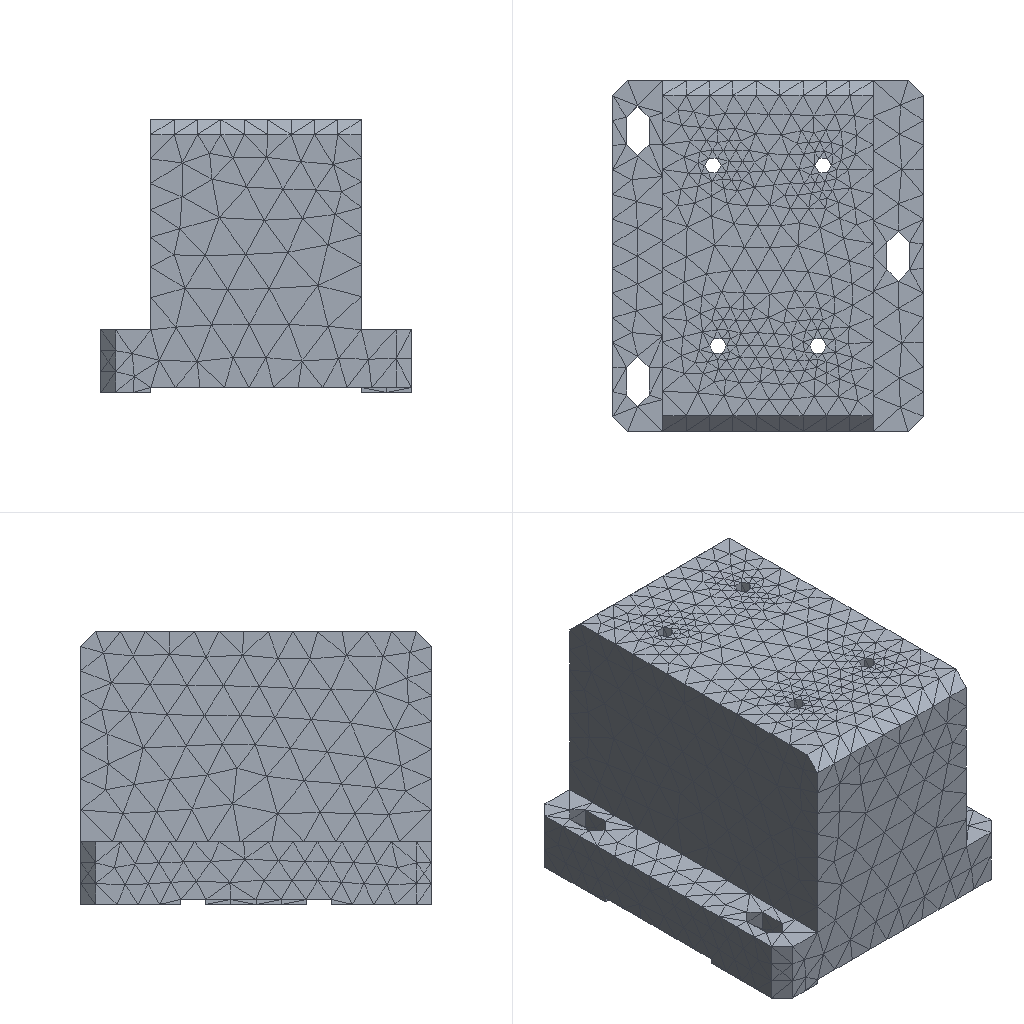Simulation study | nx simcenter
Set-up summary:
category,name,step,type,value,unit,region
solver,nx_nastran (Simcenter)
units,not stated in the deck,,not stated
analysis,deck,,static,static
analysis,solution,,SOL,101
load_step,SUBCASE 1,1,SUBCASE,SPC=1 LOAD=2
load_step,requested,,,1
mesh,nodes,,,9372
mesh,elements,,,4867
element_type,CTETRA,,solid,4867
load,nodal force total,,FX,0.0,model units
load,nodal force total,,FY,0.0,model units
load,nodal force total,,FZ,-3000000.07,model units
load,load commands in deck,,count,796
bc,support commands in deck,,count,204
analysis,NX solution 0,,Structural,Linear Statics - Single Constraint
check,setup vs results,,match,every grid point's frame and coordinates and every element id; grid points of CTETRA elements
Nastran input file, long lists of numbers shortened:
$*$$$$$$$$$$$$$$$$$$$$$$$$$$$$$$$$$$$$$$$$$$$$$$$$$$$$$$$$$$$$$$$$$
$*
$*                    NX v10.0.0.24 TRANSLATOR
$*                    FOR NX NASTRAN VERSION 10.0
$ (33 more lines like these left out)
ASSIGN OUTPUT2='131_sim1-solution_1.op2' UNIT=12
$*
$*$$$$$$$$$$$$$$$$$$$$$$$$$$$$$$$$$$$
$*
$* EXECUTIVE CONTROL
$*
$*$$$$$$$$$$$$$$$$$$$$$$$$$$$$$$$$$$$
$*
ID,NASTRAN,131_sim1-solution_1
SOL 101
CEND
$*
$*$$$$$$$$$$$$$$$$$$$$$$$$$$$$$$$$$$$
$*
$* CASE CONTROL
$*
$*$$$$$$$$$$$$$$$$$$$$$$$$$$$$$$$$$$$
$*
TITLE = Solution 1
ECHO = NONE
SPC = 1
OUTPUT
BCRESULTS(TRACTION,FORCE,PLOT) = ALL
DISPLACEMENT(PLOT) = ALL
ESE(PLOT) = ALL
FORCE(PLOT,CORNER) = ALL
OLOAD(PLOT) = ALL
SPCFORCES(PLOT) = ALL
STRAIN(PLOT,FIBER,CORNER) = ALL
STRESS(PLOT,CORNER) = ALL
$*  NX Step: Subcase - Static Loads 1
SUBCASE 1
LABEL = Subcase - Static Loads 1
LOAD = 2
$*
$*$$$$$$$$$$$$$$$$$$$$$$$$$$$$$$$$$$$
$*
$* BULK DATA
$*
$*$$$$$$$$$$$$$$$$$$$$$$$$$$$$$$$$$$$
$*
BEGIN BULK
$*
$* PARAM CARDS
$*
PARAM      K6ROT100.0000
PARAM     OIBULK     YES
PARAM    OMACHPR     YES
PARAM       POST      -2
PARAM    POSTEXT     YES
PARAM    UNITSYS   MN-MM
$*
$* GRID CARDS
$*
GRID*               9277               00.0000000000E+003.0000000000E+00+
*       0.0000000000E+00               0
GRID*               9278               0-7.234460969E-153.0000000000E+00+
*       1.2500000000E+01               0
$ (18740 more lines like these left out)
$*
$* ELEMENT CARDS
$*
$*  NX Mesh Collector: Solid(1)
$*  NX Mesh: 3d_mesh(1)
CTETRA         1       1       1       2    6003    6053     158     159+
+            160     161     162    6330
CTETRA         2       1       1       3    6003       4     163     164+
+            160     165     166     167
$ (9730 more lines like these left out)
$*
$* PROPERTY CARDS
$*
$*  NX Property: PSOLID1
PSOLID         1       1       0                           SMECH
$*
$* MATERIAL CARDS
$*
$*  NX Material: Aluminum_5086
MAT1           17.2000+7        0.3300002.6600-62.5000-5
$*
$* LOAD AND CONSTRAINT CARDS
$*
$*  NX Load and Constraint: Fixed(1)
SPC            1    4102  123456  0.0000
SPC            1    4103  123456  0.0000
SPC            1    4104  123456  0.0000
SPC            1    4105  123456  0.0000
$ (200 more lines like these left out)
$*  NX Load and Constraint: Force(1)
FORCE          2    6220       0842.4065  0.0000  0.0000-1.00000
FORCE          2    6221       0790.7649  0.0000  0.0000-1.00000
FORCE          2    6222       0 1140.00  0.0000  0.0000-1.00000
FORCE          2    6223       0812.2282  0.0000  0.0000-1.00000
$ (792 more lines like these left out)
ENDDATA 8410c588
Results summary:
result,analysis,,,static
result,last_loadstep,,,1
result,primary field,,,displacements
result,max displacement,,,0.01046,model units
result,reaction total,,FX,-0.1272,model units
result,reaction total,,FY,0.01733,model units
result,reaction total,,FZ,3000000.0,model units
result,NX solution 0,,loadcases,1,mm